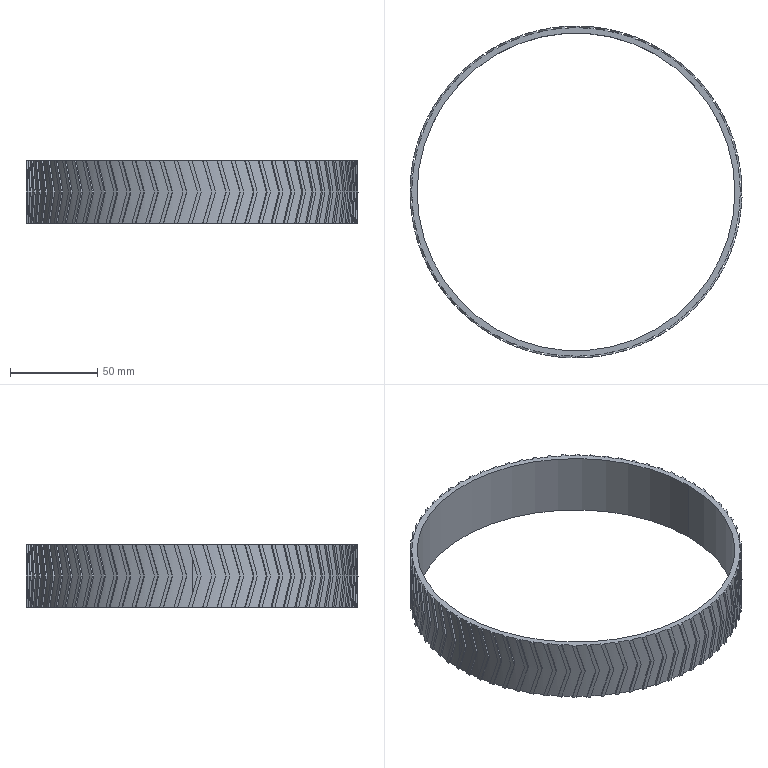Part | SolidWorks | features CirPattern 1, Extrusion 1, ICE 1 | 1 solid | 437 faces | box 190.182 x 190.182 x 36 mm | volume 68309 mm3 | plane 362 | cylinder 75 | commonest cylinder face diameters 188 x73 182 x2